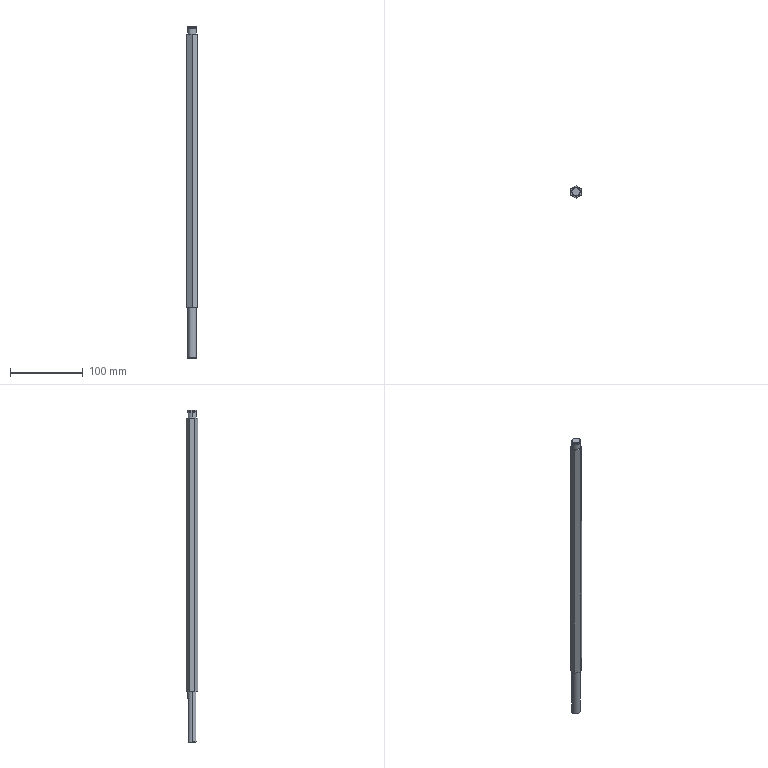Part | SolidWorks | features ICE 3, Fillet 2, Extrusion 1, RevCut 1 | 1 solid | 27 faces | box 14 x 16.166 x 456 mm | volume 72301 mm3 | plane 14 | cylinder 8 | torus 5 | commonest cylinder face diameters 12 x6 11 x2
STEP:
#1=CARTESIAN_POINT('',(-6.,0.,385.5));
#2=VERTEX_POINT('',#1);
#3=CARTESIAN_POINT('',(6.,0.,385.5));
#4=VERTEX_POINT('',#3);
#5=CARTESIAN_POINT('',(0.,0.,385.5));
#6=DIRECTION('',(0.,0.,-1.));
#7=DIRECTION('',(1.,0.,0.));
#8=AXIS2_PLACEMENT_3D('',#5,#6,#7);
#9=CIRCLE('',#8,6.);
#10=EDGE_CURVE('',#2,#4,#9,.T.);
#11=ORIENTED_EDGE('',*,*,#10,.F.);
#12=CARTESIAN_POINT('',(-5.5,0.,386.));
#13=VERTEX_POINT('',#12);
#14=CARTESIAN_POINT('',(-5.5,0.,385.5));
#15=DIRECTION('',(0.,1.,0.));
#16=DIRECTION('',(-1.,0.,0.));
#17=AXIS2_PLACEMENT_3D('',#14,#15,#16);
#18=CIRCLE('',#17,0.5);
#19=EDGE_CURVE('',#2,#13,#18,.T.);
#20=ORIENTED_EDGE('',*,*,#19,.T.);
#21=CARTESIAN_POINT('',(5.5,0.,386.));
#22=VERTEX_POINT('',#21);
#23=CARTESIAN_POINT('',(0.,0.,386.));
#24=DIRECTION('',(0.,0.,1.));
#25=DIRECTION('',(1.,0.,0.));
#26=AXIS2_PLACEMENT_3D('',#23,#24,#25);
#27=CIRCLE('',#26,5.5);
#28=EDGE_CURVE('',#22,#13,#27,.T.);
#29=ORIENTED_EDGE('',*,*,#28,.F.);
#30=CARTESIAN_POINT('',(5.5,0.,385.5));
#31=DIRECTION('',(0.,-1.,0.));
#32=DIRECTION('',(0.,0.,-1.));
#33=AXIS2_PLACEMENT_3D('',#30,#31,#32);
#34=CIRCLE('',#33,0.5);
#35=EDGE_CURVE('',#4,#22,#34,.T.);
#36=ORIENTED_EDGE('',*,*,#35,.F.);
#37=EDGE_LOOP('',(#11,#20,#29,#36));
#38=FACE_OUTER_BOUND('',#37,.T.);
#39=CARTESIAN_POINT('',(0.,0.,385.5));
#40=DIRECTION('',(0.,0.,1.));
#41=DIRECTION('',(1.,0.,0.));
#42=AXIS2_PLACEMENT_3D('',#39,#40,#41);
#43=TOROIDAL_SURFACE('',#42,5.5,0.5);
#44=ADVANCED_FACE('',(#38),#43,.T.);
#45=ORIENTED_EDGE('',*,*,#10,.T.);
#46=CARTESIAN_POINT('',(6.,0.,384.1));
#47=VERTEX_POINT('',#46);
#48=CARTESIAN_POINT('',(6.,0.,386.));
#49=DIRECTION('',(0.,0.,-1.));
#50=VECTOR('',#49,1000.);
#51=LINE('',#48,#50);
#52=EDGE_CURVE('',#4,#47,#51,.T.);
#53=ORIENTED_EDGE('',*,*,#52,.T.);
#54=CARTESIAN_POINT('',(-6.,0.,384.1));
#55=VERTEX_POINT('',#54);
#56=CARTESIAN_POINT('',(0.,0.,384.1));
#57=DIRECTION('',(0.,0.,1.));
#58=DIRECTION('',(1.,0.,0.));
#59=AXIS2_PLACEMENT_3D('',#56,#57,#58);
#60=CIRCLE('',#59,6.);
#61=EDGE_CURVE('',#47,#55,#60,.T.);
#62=ORIENTED_EDGE('',*,*,#61,.T.);
#63=CARTESIAN_POINT('',(-6.,0.,386.));
#64=DIRECTION('',(0.,0.,-1.));
#65=VECTOR('',#64,1000.);
#66=LINE('',#63,#65);
#67=EDGE_CURVE('',#2,#55,#66,.T.);
#68=ORIENTED_EDGE('',*,*,#67,.F.);
#69=EDGE_LOOP('',(#45,#53,#62,#68));
#70=FACE_OUTER_BOUND('',#69,.T.);
#71=CARTESIAN_POINT('',(0.,0.,386.));
#72=DIRECTION('',(0.,0.,-1.));
#73=DIRECTION('',(-1.,0.,0.));
#74=AXIS2_PLACEMENT_3D('',#71,#72,#73);
#75=CYLINDRICAL_SURFACE('',#74,6.);
#76=ADVANCED_FACE('',(#70),#75,.T.);
#77=CARTESIAN_POINT('',(5.5,0.,383.));
#78=VERTEX_POINT('',#77);
#79=CARTESIAN_POINT('',(-5.5,0.,383.));
#80=VERTEX_POINT('',#79);
#81=CARTESIAN_POINT('',(0.,0.,383.));
#82=DIRECTION('',(0.,0.,1.));
#83=DIRECTION('',(1.,0.,0.));
#84=AXIS2_PLACEMENT_3D('',#81,#82,#83);
#85=CIRCLE('',#84,5.5);
#86=EDGE_CURVE('',#78,#80,#85,.T.);
#87=ORIENTED_EDGE('',*,*,#86,.T.);
#88=CARTESIAN_POINT('',(-5.5,0.,384.1));
#89=VERTEX_POINT('',#88);
#90=CARTESIAN_POINT('',(-5.5,0.,418.928));
#91=DIRECTION('',(0.,0.,1.));
#92=VECTOR('',#91,1000.);
#93=LINE('',#90,#92);
#94=EDGE_CURVE('',#80,#89,#93,.T.);
#95=ORIENTED_EDGE('',*,*,#94,.T.);
#96=CARTESIAN_POINT('',(5.5,0.,384.1));
#97=VERTEX_POINT('',#96);
#98=CARTESIAN_POINT('',(0.,0.,384.1));
#99=DIRECTION('',(0.,0.,1.));
#100=DIRECTION('',(1.,0.,0.));
#101=AXIS2_PLACEMENT_3D('',#98,#99,#100);
#102=CIRCLE('',#101,5.5);
#103=EDGE_CURVE('',#97,#89,#102,.T.);
#104=ORIENTED_EDGE('',*,*,#103,.F.);
#105=CARTESIAN_POINT('',(5.5,0.,418.928));
#106=DIRECTION('',(0.,0.,1.));
#107=VECTOR('',#106,1000.);
#108=LINE('',#105,#107);
#109=EDGE_CURVE('',#78,#97,#108,.T.);
#110=ORIENTED_EDGE('',*,*,#109,.F.);
#111=EDGE_LOOP('',(#87,#95,#104,#110));
#112=FACE_OUTER_BOUND('',#111,.T.);
#113=CARTESIAN_POINT('',(0.,0.,418.928));
#114=DIRECTION('',(0.,0.,1.));
#115=DIRECTION('',(1.,0.,0.));
#116=AXIS2_PLACEMENT_3D('',#113,#114,#115);
#117=CYLINDRICAL_SURFACE('',#116,5.5);
#118=ADVANCED_FACE('',(#112),#117,.T.);
#119=CARTESIAN_POINT('',(6.,0.,-69.5));
#120=VERTEX_POINT('',#119);
#121=CARTESIAN_POINT('',(3.969,4.5,-69.5));
#122=VERTEX_POINT('',#121);
#123=CARTESIAN_POINT('',(0.,0.,-69.5));
#124=DIRECTION('',(0.,0.,1.));
#125=DIRECTION('',(-1.,0.,0.));
#126=AXIS2_PLACEMENT_3D('',#123,#124,#125);
#127=CIRCLE('',#126,6.);
#128=EDGE_CURVE('',#120,#122,#127,.T.);
#129=ORIENTED_EDGE('',*,*,#128,.F.);
#130=CARTESIAN_POINT('',(5.5,0.,-70.));
#131=VERTEX_POINT('',#130);
#132=CARTESIAN_POINT('',(5.5,0.,-69.5));
#133=DIRECTION('',(0.,1.,0.));
#134=DIRECTION('',(-1.,0.,0.));
#135=AXIS2_PLACEMENT_3D('',#132,#133,#134);
#136=CIRCLE('',#135,0.5);
#137=EDGE_CURVE('',#120,#131,#136,.T.);
#138=ORIENTED_EDGE('',*,*,#137,.T.);
#139=CARTESIAN_POINT('',(3.162,4.5,-70.));
#140=VERTEX_POINT('',#139);
#141=CARTESIAN_POINT('',(0.,0.,-70.));
#142=DIRECTION('',(0.,0.,-1.));
#143=DIRECTION('',(-1.,0.,0.));
#144=AXIS2_PLACEMENT_3D('',#141,#142,#143);
#145=CIRCLE('',#144,5.5);
#146=EDGE_CURVE('',#140,#131,#145,.T.);
#147=ORIENTED_EDGE('',*,*,#146,.F.);
#148=CARTESIAN_POINT('',(3.969,4.5,-69.5));
#149=CARTESIAN_POINT('',(3.969,4.5,-69.588));
#150=CARTESIAN_POINT('',(3.932,4.5,-69.673));
#151=CARTESIAN_POINT('',(3.819,4.5,-69.807));
#152=CARTESIAN_POINT('',(3.745,4.5,-69.858));
#153=CARTESIAN_POINT('',(3.59,4.5,-69.934));
#154=CARTESIAN_POINT('',(3.505,4.5,-69.96));
#155=CARTESIAN_POINT('',(3.335,4.5,-69.993));
#156=CARTESIAN_POINT('',(3.249,4.5,-70.));
#157=CARTESIAN_POINT('',(3.162,4.5,-70.));
#158=B_SPLINE_CURVE_WITH_KNOTS('',3,(#148,#149,#150,#151,#152,#153,#154,#155,#156,#157),.UNSPECIFIED.,.F.,.F.,(4,2,2,2,4),(0.002168,0.002429,0.00269,0.002951,0.003212),.UNSPECIFIED.);
#159=EDGE_CURVE('',#122,#140,#158,.T.);
#160=ORIENTED_EDGE('',*,*,#159,.F.);
#161=EDGE_LOOP('',(#129,#138,#147,#160));
#162=FACE_OUTER_BOUND('',#161,.T.);
#163=CARTESIAN_POINT('',(0.,0.,-69.5));
#164=DIRECTION('',(0.,0.,-1.));
#165=DIRECTION('',(-1.,0.,0.));
#166=AXIS2_PLACEMENT_3D('',#163,#164,#165);
#167=TOROIDAL_SURFACE('',#166,5.5,0.5);
#168=ADVANCED_FACE('',(#162),#167,.T.);
#169=ORIENTED_EDGE('',*,*,#137,.F.);
#170=CARTESIAN_POINT('',(-6.,0.,-69.5));
#171=VERTEX_POINT('',#170);
#172=CARTESIAN_POINT('',(0.,0.,-69.5));
#173=DIRECTION('',(0.,0.,1.));
#174=DIRECTION('',(-1.,0.,0.));
#175=AXIS2_PLACEMENT_3D('',#172,#173,#174);
#176=CIRCLE('',#175,6.);
#177=EDGE_CURVE('',#171,#120,#176,.T.);
#178=ORIENTED_EDGE('',*,*,#177,.F.);
#179=CARTESIAN_POINT('',(-5.5,0.,-70.));
#180=VERTEX_POINT('',#179);
#181=CARTESIAN_POINT('',(-5.5,0.,-69.5));
#182=DIRECTION('',(0.,-1.,0.));
#183=DIRECTION('',(0.,0.,-1.));
#184=AXIS2_PLACEMENT_3D('',#181,#182,#183);
#185=CIRCLE('',#184,0.5);
#186=EDGE_CURVE('',#171,#180,#185,.T.);
#187=ORIENTED_EDGE('',*,*,#186,.T.);
#188=CARTESIAN_POINT('',(0.,0.,-70.));
#189=DIRECTION('',(0.,0.,-1.));
#190=DIRECTION('',(-1.,0.,0.));
#191=AXIS2_PLACEMENT_3D('',#188,#189,#190);
#192=CIRCLE('',#191,5.5);
#193=EDGE_CURVE('',#131,#180,#192,.T.);
#194=ORIENTED_EDGE('',*,*,#193,.F.);
#195=EDGE_LOOP('',(#169,#178,#187,#194));
#196=FACE_OUTER_BOUND('',#195,.T.);
#197=CARTESIAN_POINT('',(0.,0.,-69.5));
#198=DIRECTION('',(0.,0.,-1.));
#199=DIRECTION('',(-1.,0.,0.));
#200=AXIS2_PLACEMENT_3D('',#197,#198,#199);
#201=TOROIDAL_SURFACE('',#200,5.5,0.5);
#202=ADVANCED_FACE('',(#196),#201,.T.);
#203=CARTESIAN_POINT('',(-3.969,4.5,-69.5));
#204=VERTEX_POINT('',#203);
#205=CARTESIAN_POINT('',(0.,0.,-69.5));
#206=DIRECTION('',(0.,0.,1.));
#207=DIRECTION('',(-1.,0.,0.));
#208=AXIS2_PLACEMENT_3D('',#205,#206,#207);
#209=CIRCLE('',#208,6.);
#210=EDGE_CURVE('',#204,#171,#209,.T.);
#211=ORIENTED_EDGE('',*,*,#210,.T.);
#212=CARTESIAN_POINT('',(-6.,0.,0.));
#213=VERTEX_POINT('',#212);
#214=CARTESIAN_POINT('',(-6.,0.,-70.));
#215=DIRECTION('',(0.,0.,1.));
#216=VECTOR('',#215,1000.);
#217=LINE('',#214,#216);
#218=EDGE_CURVE('',#171,#213,#217,.T.);
#219=ORIENTED_EDGE('',*,*,#218,.T.);
#220=CARTESIAN_POINT('',(6.,0.,0.));
#221=VERTEX_POINT('',#220);
#222=CARTESIAN_POINT('',(0.,0.,0.));
#223=DIRECTION('',(0.,0.,-1.));
#224=DIRECTION('',(1.,0.,0.));
#225=AXIS2_PLACEMENT_3D('',#222,#223,#224);
#226=CIRCLE('',#225,6.);
#227=EDGE_CURVE('',#213,#221,#226,.T.);
#228=ORIENTED_EDGE('',*,*,#227,.T.);
#229=CARTESIAN_POINT('',(6.,0.,-70.));
#230=DIRECTION('',(0.,0.,1.));
#231=VECTOR('',#230,1000.);
#232=LINE('',#229,#231);
#233=EDGE_CURVE('',#120,#221,#232,.T.);
#234=ORIENTED_EDGE('',*,*,#233,.F.);
#235=ORIENTED_EDGE('',*,*,#128,.T.);
#236=CARTESIAN_POINT('',(3.969,4.5,-10.));
#237=VERTEX_POINT('',#236);
#238=CARTESIAN_POINT('',(3.969,4.5,-70.));
#239=DIRECTION('',(0.,0.,1.));
#240=VECTOR('',#239,1000.);
#241=LINE('',#238,#240);
#242=EDGE_CURVE('',#122,#237,#241,.T.);
#243=ORIENTED_EDGE('',*,*,#242,.T.);
#244=CARTESIAN_POINT('',(-3.969,4.5,-10.));
#245=VERTEX_POINT('',#244);
#246=CARTESIAN_POINT('',(0.,0.,-10.));
#247=DIRECTION('',(0.,0.,1.));
#248=DIRECTION('',(1.,0.,0.));
#249=AXIS2_PLACEMENT_3D('',#246,#247,#248);
#250=CIRCLE('',#249,6.);
#251=EDGE_CURVE('',#237,#245,#250,.T.);
#252=ORIENTED_EDGE('',*,*,#251,.T.);
#253=CARTESIAN_POINT('',(-3.969,4.5,-70.));
#254=DIRECTION('',(0.,0.,-1.));
#255=VECTOR('',#254,1000.);
#256=LINE('',#253,#255);
#257=EDGE_CURVE('',#245,#204,#256,.T.);
#258=ORIENTED_EDGE('',*,*,#257,.T.);
#259=EDGE_LOOP('',(#211,#219,#228,#234,#235,#243,#252,#258));
#260=FACE_OUTER_BOUND('',#259,.T.);
#261=CARTESIAN_POINT('',(0.,0.,-70.));
#262=DIRECTION('',(0.,0.,1.));
#263=DIRECTION('',(1.,0.,0.));
#264=AXIS2_PLACEMENT_3D('',#261,#262,#263);
#265=CYLINDRICAL_SURFACE('',#264,6.);
#266=ADVANCED_FACE('',(#260),#265,.T.);
#267=CARTESIAN_POINT('',(-6.,0.,383.));
#268=VERTEX_POINT('',#267);
#269=CARTESIAN_POINT('',(6.,0.,383.));
#270=VERTEX_POINT('',#269);
#271=CARTESIAN_POINT('',(0.,0.,383.));
#272=DIRECTION('',(0.,0.,-1.));
#273=DIRECTION('',(-1.,0.,0.));
#274=AXIS2_PLACEMENT_3D('',#271,#272,#273);
#275=CIRCLE('',#274,6.);
#276=EDGE_CURVE('',#268,#270,#275,.T.);
#277=ORIENTED_EDGE('',*,*,#276,.T.);
#278=CARTESIAN_POINT('',(6.,0.,375.));
#279=VERTEX_POINT('',#278);
#280=CARTESIAN_POINT('',(6.,0.,386.));
#281=DIRECTION('',(0.,0.,-1.));
#282=VECTOR('',#281,1000.);
#283=LINE('',#280,#282);
#284=EDGE_CURVE('',#270,#279,#283,.T.);
#285=ORIENTED_EDGE('',*,*,#284,.T.);
#286=CARTESIAN_POINT('',(-6.,0.,375.));
#287=VERTEX_POINT('',#286);
#288=CARTESIAN_POINT('',(0.,0.,375.));
#289=DIRECTION('',(0.,0.,1.));
#290=DIRECTION('',(1.,0.,0.));
#291=AXIS2_PLACEMENT_3D('',#288,#289,#290);
#292=CIRCLE('',#291,6.);
#293=EDGE_CURVE('',#279,#287,#292,.T.);
#294=ORIENTED_EDGE('',*,*,#293,.T.);
#295=CARTESIAN_POINT('',(-6.,0.,386.));
#296=DIRECTION('',(0.,0.,-1.));
#297=VECTOR('',#296,1000.);
#298=LINE('',#295,#297);
#299=EDGE_CURVE('',#268,#287,#298,.T.);
#300=ORIENTED_EDGE('',*,*,#299,.F.);
#301=EDGE_LOOP('',(#277,#285,#294,#300));
#302=FACE_OUTER_BOUND('',#301,.T.);
#303=CARTESIAN_POINT('',(0.,0.,386.));
#304=DIRECTION('',(0.,0.,-1.));
#305=DIRECTION('',(-1.,0.,0.));
#306=AXIS2_PLACEMENT_3D('',#303,#304,#305);
#307=CYLINDRICAL_SURFACE('',#306,6.);
#308=ADVANCED_FACE('',(#302),#307,.T.);
#309=ORIENTED_EDGE('',*,*,#284,.F.);
#310=CARTESIAN_POINT('',(0.,0.,383.));
#311=DIRECTION('',(0.,0.,-1.));
#312=DIRECTION('',(-1.,0.,0.));
#313=AXIS2_PLACEMENT_3D('',#310,#311,#312);
#314=CIRCLE('',#313,6.);
#315=EDGE_CURVE('',#270,#268,#314,.T.);
#316=ORIENTED_EDGE('',*,*,#315,.T.);
#317=ORIENTED_EDGE('',*,*,#299,.T.);
#318=CARTESIAN_POINT('',(0.,0.,375.));
#319=DIRECTION('',(0.,0.,1.));
#320=DIRECTION('',(1.,0.,0.));
#321=AXIS2_PLACEMENT_3D('',#318,#319,#320);
#322=CIRCLE('',#321,6.);
#323=EDGE_CURVE('',#287,#279,#322,.T.);
#324=ORIENTED_EDGE('',*,*,#323,.T.);
#325=EDGE_LOOP('',(#309,#316,#317,#324));
#326=FACE_OUTER_BOUND('',#325,.T.);
#327=CARTESIAN_POINT('',(0.,0.,386.));
#328=DIRECTION('',(0.,0.,-1.));
#329=DIRECTION('',(-1.,0.,0.));
#330=AXIS2_PLACEMENT_3D('',#327,#328,#329);
#331=CYLINDRICAL_SURFACE('',#330,6.);
#332=ADVANCED_FACE('',(#326),#331,.T.);
#333=CARTESIAN_POINT('',(0.,-8.083,375.));
#334=VERTEX_POINT('',#333);
#335=CARTESIAN_POINT('',(7.,-4.041,375.));
#336=VERTEX_POINT('',#335);
#337=CARTESIAN_POINT('',(0.,-8.083,375.));
#338=DIRECTION('',(0.866,0.5,0.));
#339=VECTOR('',#338,1000.);
#340=LINE('',#337,#339);
#341=EDGE_CURVE('',#334,#336,#340,.T.);
#342=ORIENTED_EDGE('',*,*,#341,.T.);
#343=CARTESIAN_POINT('',(7.,4.041,375.));
#344=VERTEX_POINT('',#343);
#345=CARTESIAN_POINT('',(7.,-4.041,375.));
#346=DIRECTION('',(0.,1.,0.));
#347=VECTOR('',#346,1000.);
#348=LINE('',#345,#347);
#349=EDGE_CURVE('',#336,#344,#348,.T.);
#350=ORIENTED_EDGE('',*,*,#349,.T.);
#351=CARTESIAN_POINT('',(0.,8.083,375.));
#352=VERTEX_POINT('',#351);
#353=CARTESIAN_POINT('',(7.,4.041,375.));
#354=DIRECTION('',(-0.866,0.5,0.));
#355=VECTOR('',#354,1000.);
#356=LINE('',#353,#355);
#357=EDGE_CURVE('',#344,#352,#356,.T.);
#358=ORIENTED_EDGE('',*,*,#357,.T.);
#359=CARTESIAN_POINT('',(-7.,4.041,375.));
#360=VERTEX_POINT('',#359);
#361=CARTESIAN_POINT('',(0.,8.083,375.));
#362=DIRECTION('',(-0.866,-0.5,0.));
#363=VECTOR('',#362,1000.);
#364=LINE('',#361,#363);
#365=EDGE_CURVE('',#352,#360,#364,.T.);
#366=ORIENTED_EDGE('',*,*,#365,.T.);
#367=CARTESIAN_POINT('',(-7.,-4.041,375.));
#368=VERTEX_POINT('',#367);
#369=CARTESIAN_POINT('',(-7.,4.041,375.));
#370=DIRECTION('',(0.,-1.,0.));
#371=VECTOR('',#370,1000.);
#372=LINE('',#369,#371);
#373=EDGE_CURVE('',#360,#368,#372,.T.);
#374=ORIENTED_EDGE('',*,*,#373,.T.);
#375=CARTESIAN_POINT('',(-7.,-4.041,375.));
#376=DIRECTION('',(0.866,-0.5,0.));
#377=VECTOR('',#376,1000.);
#378=LINE('',#375,#377);
#379=EDGE_CURVE('',#368,#334,#378,.T.);
#380=ORIENTED_EDGE('',*,*,#379,.T.);
#381=EDGE_LOOP('',(#342,#350,#358,#366,#374,#380));
#382=FACE_OUTER_BOUND('',#381,.T.);
#383=ORIENTED_EDGE('',*,*,#323,.F.);
#384=ORIENTED_EDGE('',*,*,#293,.F.);
#385=EDGE_LOOP('',(#383,#384));
#386=FACE_BOUND('',#385,.T.);
#387=CARTESIAN_POINT('',(0.,0.,375.));
#388=DIRECTION('',(0.,0.,1.));
#389=DIRECTION('',(1.,0.,0.));
#390=AXIS2_PLACEMENT_3D('',#387,#388,#389);
#391=PLANE('',#390);
#392=ADVANCED_FACE('',(#382,#386),#391,.T.);
#393=CARTESIAN_POINT('',(0.,-8.083,0.));
#394=VERTEX_POINT('',#393);
#395=CARTESIAN_POINT('',(7.,-4.041,0.));
#396=VERTEX_POINT('',#395);
#397=CARTESIAN_POINT('',(0.,-8.083,0.));
#398=DIRECTION('',(0.866,0.5,0.));
#399=VECTOR('',#398,1000.);
#400=LINE('',#397,#399);
#401=EDGE_CURVE('',#394,#396,#400,.T.);
#402=ORIENTED_EDGE('',*,*,#401,.F.);
#403=CARTESIAN_POINT('',(-7.,-4.041,0.));
#404=VERTEX_POINT('',#403);
#405=CARTESIAN_POINT('',(-7.,-4.041,0.));
#406=DIRECTION('',(0.866,-0.5,0.));
#407=VECTOR('',#406,1000.);
#408=LINE('',#405,#407);
#409=EDGE_CURVE('',#404,#394,#408,.T.);
#410=ORIENTED_EDGE('',*,*,#409,.F.);
#411=CARTESIAN_POINT('',(-7.,4.041,0.));
#412=VERTEX_POINT('',#411);
#413=CARTESIAN_POINT('',(-7.,4.041,0.));
#414=DIRECTION('',(0.,-1.,0.));
#415=VECTOR('',#414,1000.);
#416=LINE('',#413,#415);
#417=EDGE_CURVE('',#412,#404,#416,.T.);
#418=ORIENTED_EDGE('',*,*,#417,.F.);
#419=CARTESIAN_POINT('',(0.,8.083,0.));
#420=VERTEX_POINT('',#419);
#421=CARTESIAN_POINT('',(0.,8.083,0.));
#422=DIRECTION('',(-0.866,-0.5,0.));
#423=VECTOR('',#422,1000.);
#424=LINE('',#421,#423);
#425=EDGE_CURVE('',#420,#412,#424,.T.);
#426=ORIENTED_EDGE('',*,*,#425,.F.);
#427=CARTESIAN_POINT('',(7.,4.041,0.));
#428=VERTEX_POINT('',#427);
#429=CARTESIAN_POINT('',(7.,4.041,0.));
#430=DIRECTION('',(-0.866,0.5,0.));
#431=VECTOR('',#430,1000.);
#432=LINE('',#429,#431);
#433=EDGE_CURVE('',#428,#420,#432,.T.);
#434=ORIENTED_EDGE('',*,*,#433,.F.);
#435=CARTESIAN_POINT('',(7.,-4.041,0.));
#436=DIRECTION('',(0.,1.,0.));
#437=VECTOR('',#436,1000.);
#438=LINE('',#435,#437);
#439=EDGE_CURVE('',#396,#428,#438,.T.);
#440=ORIENTED_EDGE('',*,*,#439,.F.);
#441=EDGE_LOOP('',(#402,#410,#418,#426,#434,#440));
#442=FACE_OUTER_BOUND('',#441,.T.);
#443=CARTESIAN_POINT('',(0.,0.,0.));
#444=DIRECTION('',(0.,0.,-1.));
#445=DIRECTION('',(1.,0.,0.));
#446=AXIS2_PLACEMENT_3D('',#443,#444,#445);
#447=CIRCLE('',#446,6.);
#448=EDGE_CURVE('',#221,#213,#447,.T.);
#449=ORIENTED_EDGE('',*,*,#448,.F.);
#450=ORIENTED_EDGE('',*,*,#227,.F.);
#451=EDGE_LOOP('',(#449,#450));
#452=FACE_BOUND('',#451,.T.);
#453=CARTESIAN_POINT('',(0.,0.,0.));
#454=DIRECTION('',(0.,0.,1.));
#455=DIRECTION('',(1.,0.,0.));
#456=AXIS2_PLACEMENT_3D('',#453,#454,#455);
#457=PLANE('',#456);
#458=ADVANCED_FACE('',(#442,#452),#457,.F.);
#459=ORIENTED_EDGE('',*,*,#401,.T.);
#460=CARTESIAN_POINT('',(7.,-4.041,375.));
#461=DIRECTION('',(0.,0.,-1.));
#462=VECTOR('',#461,1000.);
#463=LINE('',#460,#462);
#464=EDGE_CURVE('',#336,#396,#463,.T.);
#465=ORIENTED_EDGE('',*,*,#464,.F.);
#466=ORIENTED_EDGE('',*,*,#341,.F.);
#467=CARTESIAN_POINT('',(0.,-8.083,375.));
#468=DIRECTION('',(0.,0.,-1.));
#469=VECTOR('',#468,1000.);
#470=LINE('',#467,#469);
#471=EDGE_CURVE('',#334,#394,#470,.T.);
#472=ORIENTED_EDGE('',*,*,#471,.T.);
#473=EDGE_LOOP('',(#459,#465,#466,#472));
#474=FACE_OUTER_BOUND('',#473,.T.);
#475=CARTESIAN_POINT('',(0.,-8.083,375.));
#476=DIRECTION('',(-0.5,0.866,0.));
#477=DIRECTION('',(-0.866,-0.5,0.));
#478=AXIS2_PLACEMENT_3D('',#475,#476,#477);
#479=PLANE('',#478);
#480=ADVANCED_FACE('',(#474),#479,.F.);
#481=ORIENTED_EDGE('',*,*,#439,.T.);
#482=CARTESIAN_POINT('',(7.,4.041,375.));
#483=DIRECTION('',(0.,0.,-1.));
#484=VECTOR('',#483,1000.);
#485=LINE('',#482,#484);
#486=EDGE_CURVE('',#344,#428,#485,.T.);
#487=ORIENTED_EDGE('',*,*,#486,.F.);
#488=ORIENTED_EDGE('',*,*,#349,.F.);
#489=ORIENTED_EDGE('',*,*,#464,.T.);
#490=EDGE_LOOP('',(#481,#487,#488,#489));
#491=FACE_OUTER_BOUND('',#490,.T.);
#492=CARTESIAN_POINT('',(7.,-4.041,375.));
#493=DIRECTION('',(-1.,0.,0.));
#494=DIRECTION('',(0.,-1.,0.));
#495=AXIS2_PLACEMENT_3D('',#492,#493,#494);
#496=PLANE('',#495);
#497=ADVANCED_FACE('',(#491),#496,.F.);
#498=ORIENTED_EDGE('',*,*,#433,.T.);
#499=CARTESIAN_POINT('',(0.,8.083,375.));
#500=DIRECTION('',(0.,0.,-1.));
#501=VECTOR('',#500,1000.);
#502=LINE('',#499,#501);
#503=EDGE_CURVE('',#352,#420,#502,.T.);
#504=ORIENTED_EDGE('',*,*,#503,.F.);
#505=ORIENTED_EDGE('',*,*,#357,.F.);
#506=ORIENTED_EDGE('',*,*,#486,.T.);
#507=EDGE_LOOP('',(#498,#504,#505,#506));
#508=FACE_OUTER_BOUND('',#507,.T.);
#509=CARTESIAN_POINT('',(7.,4.041,375.));
#510=DIRECTION('',(-0.5,-0.866,0.));
#511=DIRECTION('',(0.866,-0.5,0.));
#512=AXIS2_PLACEMENT_3D('',#509,#510,#511);
#513=PLANE('',#512);
#514=ADVANCED_FACE('',(#508),#513,.F.);
#515=ORIENTED_EDGE('',*,*,#425,.T.);
#516=CARTESIAN_POINT('',(-7.,4.041,375.));
#517=DIRECTION('',(0.,0.,-1.));
#518=VECTOR('',#517,1000.);
#519=LINE('',#516,#518);
#520=EDGE_CURVE('',#360,#412,#519,.T.);
#521=ORIENTED_EDGE('',*,*,#520,.F.);
#522=ORIENTED_EDGE('',*,*,#365,.F.);
#523=ORIENTED_EDGE('',*,*,#503,.T.);
#524=EDGE_LOOP('',(#515,#521,#522,#523));
#525=FACE_OUTER_BOUND('',#524,.T.);
#526=CARTESIAN_POINT('',(0.,8.083,375.));
#527=DIRECTION('',(0.5,-0.866,0.));
#528=DIRECTION('',(0.866,0.5,0.));
#529=AXIS2_PLACEMENT_3D('',#526,#527,#528);
#530=PLANE('',#529);
#531=ADVANCED_FACE('',(#525),#530,.F.);
#532=ORIENTED_EDGE('',*,*,#417,.T.);
#533=CARTESIAN_POINT('',(-7.,-4.041,375.));
#534=DIRECTION('',(0.,0.,-1.));
#535=VECTOR('',#534,1000.);
#536=LINE('',#533,#535);
#537=EDGE_CURVE('',#368,#404,#536,.T.);
#538=ORIENTED_EDGE('',*,*,#537,.F.);
#539=ORIENTED_EDGE('',*,*,#373,.F.);
#540=ORIENTED_EDGE('',*,*,#520,.T.);
#541=EDGE_LOOP('',(#532,#538,#539,#540));
#542=FACE_OUTER_BOUND('',#541,.T.);
#543=CARTESIAN_POINT('',(-7.,4.041,375.));
#544=DIRECTION('',(1.,0.,0.));
#545=DIRECTION('',(0.,1.,0.));
#546=AXIS2_PLACEMENT_3D('',#543,#544,#545);
#547=PLANE('',#546);
#548=ADVANCED_FACE('',(#542),#547,.F.);
#549=ORIENTED_EDGE('',*,*,#409,.T.);
#550=ORIENTED_EDGE('',*,*,#471,.F.);
#551=ORIENTED_EDGE('',*,*,#379,.F.);
#552=ORIENTED_EDGE('',*,*,#537,.T.);
#553=EDGE_LOOP('',(#549,#550,#551,#552));
#554=FACE_OUTER_BOUND('',#553,.T.);
#555=CARTESIAN_POINT('',(-7.,-4.041,375.));
#556=DIRECTION('',(0.5,0.866,0.));
#557=DIRECTION('',(-0.866,0.5,0.));
#558=AXIS2_PLACEMENT_3D('',#555,#556,#557);
#559=PLANE('',#558);
#560=ADVANCED_FACE('',(#554),#559,.F.);
#561=ORIENTED_EDGE('',*,*,#218,.F.);
#562=ORIENTED_EDGE('',*,*,#177,.T.);
#563=ORIENTED_EDGE('',*,*,#233,.T.);
#564=ORIENTED_EDGE('',*,*,#448,.T.);
#565=EDGE_LOOP('',(#561,#562,#563,#564));
#566=FACE_OUTER_BOUND('',#565,.T.);
#567=CARTESIAN_POINT('',(0.,0.,-70.));
#568=DIRECTION('',(0.,0.,1.));
#569=DIRECTION('',(1.,0.,0.));
#570=AXIS2_PLACEMENT_3D('',#567,#568,#569);
#571=CYLINDRICAL_SURFACE('',#570,6.);
#572=ADVANCED_FACE('',(#566),#571,.T.);
#573=CARTESIAN_POINT('',(-3.162,4.5,-70.));
#574=VERTEX_POINT('',#573);
#575=CARTESIAN_POINT('',(-5.,4.5,-70.));
#576=DIRECTION('',(-1.,0.,0.));
#577=VECTOR('',#576,1000.);
#578=LINE('',#575,#577);
#579=EDGE_CURVE('',#140,#574,#578,.T.);
#580=ORIENTED_EDGE('',*,*,#579,.F.);
#581=ORIENTED_EDGE('',*,*,#146,.T.);
#582=ORIENTED_EDGE('',*,*,#193,.T.);
#583=CARTESIAN_POINT('',(0.,0.,-70.));
#584=DIRECTION('',(0.,0.,-1.));
#585=DIRECTION('',(-1.,0.,0.));
#586=AXIS2_PLACEMENT_3D('',#583,#584,#585);
#587=CIRCLE('',#586,5.5);
#588=EDGE_CURVE('',#180,#574,#587,.T.);
#589=ORIENTED_EDGE('',*,*,#588,.T.);
#590=EDGE_LOOP('',(#580,#581,#582,#589));
#591=FACE_OUTER_BOUND('',#590,.T.);
#592=CARTESIAN_POINT('',(0.,0.,-70.));
#593=DIRECTION('',(0.,0.,-1.));
#594=DIRECTION('',(-1.,0.,0.));
#595=AXIS2_PLACEMENT_3D('',#592,#593,#594);
#596=PLANE('',#595);
#597=ADVANCED_FACE('',(#591),#596,.T.);
#598=ORIENTED_EDGE('',*,*,#186,.F.);
#599=ORIENTED_EDGE('',*,*,#210,.F.);
#600=CARTESIAN_POINT('',(-3.162,4.5,-70.));
#601=CARTESIAN_POINT('',(-3.335,4.5,-70.));
#602=CARTESIAN_POINT('',(-3.512,4.5,-69.972));
#603=CARTESIAN_POINT('',(-3.747,4.5,-69.857));
#604=CARTESIAN_POINT('',(-3.82,4.5,-69.806));
#605=CARTESIAN_POINT('',(-3.931,4.5,-69.673));
#606=CARTESIAN_POINT('',(-3.969,4.5,-69.587));
#607=CARTESIAN_POINT('',(-3.969,4.5,-69.5));
#608=B_SPLINE_CURVE_WITH_KNOTS('',3,(#600,#601,#602,#603,#604,#605,#606,#607),.UNSPECIFIED.,.F.,.F.,(4,2,2,4),(0.003478,0.004,0.004262,0.004523),.UNSPECIFIED.);
#609=EDGE_CURVE('',#574,#204,#608,.T.);
#610=ORIENTED_EDGE('',*,*,#609,.F.);
#611=ORIENTED_EDGE('',*,*,#588,.F.);
#612=EDGE_LOOP('',(#598,#599,#610,#611));
#613=FACE_OUTER_BOUND('',#612,.T.);
#614=CARTESIAN_POINT('',(0.,0.,-69.5));
#615=DIRECTION('',(0.,0.,-1.));
#616=DIRECTION('',(-1.,0.,0.));
#617=AXIS2_PLACEMENT_3D('',#614,#615,#616);
#618=TOROIDAL_SURFACE('',#617,5.5,0.5);
#619=ADVANCED_FACE('',(#613),#618,.T.);
#620=ORIENTED_EDGE('',*,*,#86,.F.);
#621=CARTESIAN_POINT('',(0.,0.,383.));
#622=DIRECTION('',(0.,0.,1.));
#623=DIRECTION('',(1.,0.,0.));
#624=AXIS2_PLACEMENT_3D('',#621,#622,#623);
#625=CIRCLE('',#624,5.5);
#626=EDGE_CURVE('',#80,#78,#625,.T.);
#627=ORIENTED_EDGE('',*,*,#626,.F.);
#628=EDGE_LOOP('',(#620,#627));
#629=FACE_BOUND('',#628,.T.);
#630=ORIENTED_EDGE('',*,*,#276,.F.);
#631=ORIENTED_EDGE('',*,*,#315,.F.);
#632=EDGE_LOOP('',(#630,#631));
#633=FACE_OUTER_BOUND('',#632,.T.);
#634=CARTESIAN_POINT('',(5.5,0.,383.));
#635=DIRECTION('',(0.,0.,-1.));
#636=DIRECTION('',(-1.,0.,0.));
#637=AXIS2_PLACEMENT_3D('',#634,#635,#636);
#638=PLANE('',#637);
#639=ADVANCED_FACE('',(#629,#633),#638,.F.);
#640=ORIENTED_EDGE('',*,*,#103,.T.);
#641=CARTESIAN_POINT('',(0.,0.,384.1));
#642=DIRECTION('',(0.,0.,1.));
#643=DIRECTION('',(1.,0.,0.));
#644=AXIS2_PLACEMENT_3D('',#641,#642,#643);
#645=CIRCLE('',#644,5.5);
#646=EDGE_CURVE('',#89,#97,#645,.T.);
#647=ORIENTED_EDGE('',*,*,#646,.T.);
#648=EDGE_LOOP('',(#640,#647));
#649=FACE_BOUND('',#648,.T.);
#650=CARTESIAN_POINT('',(0.,0.,384.1));
#651=DIRECTION('',(0.,0.,1.));
#652=DIRECTION('',(1.,0.,0.));
#653=AXIS2_PLACEMENT_3D('',#650,#651,#652);
#654=CIRCLE('',#653,6.);
#655=EDGE_CURVE('',#55,#47,#654,.T.);
#656=ORIENTED_EDGE('',*,*,#655,.F.);
#657=ORIENTED_EDGE('',*,*,#61,.F.);
#658=EDGE_LOOP('',(#656,#657));
#659=FACE_OUTER_BOUND('',#658,.T.);
#660=CARTESIAN_POINT('',(5.5,0.,384.1));
#661=DIRECTION('',(0.,0.,1.));
#662=DIRECTION('',(1.,0.,0.));
#663=AXIS2_PLACEMENT_3D('',#660,#661,#662);
#664=PLANE('',#663);
#665=ADVANCED_FACE('',(#649,#659),#664,.F.);
#666=ORIENTED_EDGE('',*,*,#94,.F.);
#667=ORIENTED_EDGE('',*,*,#626,.T.);
#668=ORIENTED_EDGE('',*,*,#109,.T.);
#669=ORIENTED_EDGE('',*,*,#646,.F.);
#670=EDGE_LOOP('',(#666,#667,#668,#669));
#671=FACE_OUTER_BOUND('',#670,.T.);
#672=CARTESIAN_POINT('',(0.,0.,418.928));
#673=DIRECTION('',(0.,0.,1.));
#674=DIRECTION('',(1.,0.,0.));
#675=AXIS2_PLACEMENT_3D('',#672,#673,#674);
#676=CYLINDRICAL_SURFACE('',#675,5.5);
#677=ADVANCED_FACE('',(#671),#676,.T.);
#678=ORIENTED_EDGE('',*,*,#28,.T.);
#679=CARTESIAN_POINT('',(0.,0.,386.));
#680=DIRECTION('',(0.,0.,1.));
#681=DIRECTION('',(1.,0.,0.));
#682=AXIS2_PLACEMENT_3D('',#679,#680,#681);
#683=CIRCLE('',#682,5.5);
#684=EDGE_CURVE('',#13,#22,#683,.T.);
#685=ORIENTED_EDGE('',*,*,#684,.T.);
#686=EDGE_LOOP('',(#678,#685));
#687=FACE_OUTER_BOUND('',#686,.T.);
#688=CARTESIAN_POINT('',(0.,0.,386.));
#689=DIRECTION('',(0.,0.,1.));
#690=DIRECTION('',(1.,0.,0.));
#691=AXIS2_PLACEMENT_3D('',#688,#689,#690);
#692=PLANE('',#691);
#693=ADVANCED_FACE('',(#687),#692,.T.);
#694=ORIENTED_EDGE('',*,*,#52,.F.);
#695=CARTESIAN_POINT('',(0.,0.,385.5));
#696=DIRECTION('',(0.,0.,-1.));
#697=DIRECTION('',(1.,0.,0.));
#698=AXIS2_PLACEMENT_3D('',#695,#696,#697);
#699=CIRCLE('',#698,6.);
#700=EDGE_CURVE('',#4,#2,#699,.T.);
#701=ORIENTED_EDGE('',*,*,#700,.T.);
#702=ORIENTED_EDGE('',*,*,#67,.T.);
#703=ORIENTED_EDGE('',*,*,#655,.T.);
#704=EDGE_LOOP('',(#694,#701,#702,#703));
#705=FACE_OUTER_BOUND('',#704,.T.);
#706=CARTESIAN_POINT('',(0.,0.,386.));
#707=DIRECTION('',(0.,0.,-1.));
#708=DIRECTION('',(-1.,0.,0.));
#709=AXIS2_PLACEMENT_3D('',#706,#707,#708);
#710=CYLINDRICAL_SURFACE('',#709,6.);
#711=ADVANCED_FACE('',(#705),#710,.T.);
#712=ORIENTED_EDGE('',*,*,#19,.F.);
#713=ORIENTED_EDGE('',*,*,#700,.F.);
#714=ORIENTED_EDGE('',*,*,#35,.T.);
#715=ORIENTED_EDGE('',*,*,#684,.F.);
#716=EDGE_LOOP('',(#712,#713,#714,#715));
#717=FACE_OUTER_BOUND('',#716,.T.);
#718=CARTESIAN_POINT('',(0.,0.,385.5));
#719=DIRECTION('',(0.,0.,1.));
#720=DIRECTION('',(1.,0.,0.));
#721=AXIS2_PLACEMENT_3D('',#718,#719,#720);
#722=TOROIDAL_SURFACE('',#721,5.5,0.5);
#723=ADVANCED_FACE('',(#717),#722,.T.);
#724=CARTESIAN_POINT('',(-5.,4.5,-10.));
#725=DIRECTION('',(-1.,0.,0.));
#726=VECTOR('',#725,1000.);
#727=LINE('',#724,#726);
#728=EDGE_CURVE('',#237,#245,#727,.T.);
#729=ORIENTED_EDGE('',*,*,#728,.T.);
#730=ORIENTED_EDGE('',*,*,#251,.F.);
#731=EDGE_LOOP('',(#729,#730));
#732=FACE_OUTER_BOUND('',#731,.T.);
#733=CARTESIAN_POINT('',(0.,0.,-10.));
#734=DIRECTION('',(0.,0.,1.));
#735=DIRECTION('',(1.,0.,0.));
#736=AXIS2_PLACEMENT_3D('',#733,#734,#735);
#737=PLANE('',#736);
#738=ADVANCED_FACE('',(#732),#737,.F.);
#739=ORIENTED_EDGE('',*,*,#728,.F.);
#740=ORIENTED_EDGE('',*,*,#242,.F.);
#741=ORIENTED_EDGE('',*,*,#159,.T.);
#742=ORIENTED_EDGE('',*,*,#579,.T.);
#743=ORIENTED_EDGE('',*,*,#609,.T.);
#744=ORIENTED_EDGE('',*,*,#257,.F.);
#745=EDGE_LOOP('',(#739,#740,#741,#742,#743,#744));
#746=FACE_OUTER_BOUND('',#745,.T.);
#747=CARTESIAN_POINT('',(-5.,4.5,-10.));
#748=DIRECTION('',(0.,-1.,0.));
#749=DIRECTION('',(1.,0.,0.));
#750=AXIS2_PLACEMENT_3D('',#747,#748,#749);
#751=PLANE('',#750);
#752=ADVANCED_FACE('',(#746),#751,.F.);
#753=CLOSED_SHELL('',(#44,#76,#118,#168,#202,#266,#308,#332,#392,#458,#480,#497,#514,#531,#548,#560,#572,#597,#619,#639,#665,#677,#693,#711,#723,#738,#752));
#754=MANIFOLD_SOLID_BREP('',#753);
#755=CARTESIAN_POINT('',(0.,0.,0.));
#756=DIRECTION('',(0.,0.,1.));
#757=DIRECTION('',(1.,0.,0.));
#758=AXIS2_PLACEMENT_3D('',#755,#756,#757);
#759=(LENGTH_UNIT()NAMED_UNIT(*)SI_UNIT(.MILLI.,.METRE.));
#760=UNCERTAINTY_MEASURE_WITH_UNIT(LENGTH_MEASURE(0.00001),#759,'','');
#761=(NAMED_UNIT(*)PLANE_ANGLE_UNIT()SI_UNIT($,.RADIAN.));
#762=(NAMED_UNIT(*)SI_UNIT($,.STERADIAN.)SOLID_ANGLE_UNIT());
#763=(GEOMETRIC_REPRESENTATION_CONTEXT(3)GLOBAL_UNCERTAINTY_ASSIGNED_CONTEXT((#760))GLOBAL_UNIT_ASSIGNED_CONTEXT((#759,#761,#762))REPRESENTATION_CONTEXT('',''));
#764=ADVANCED_BREP_SHAPE_REPRESENTATION('',(#754,#758),#763);